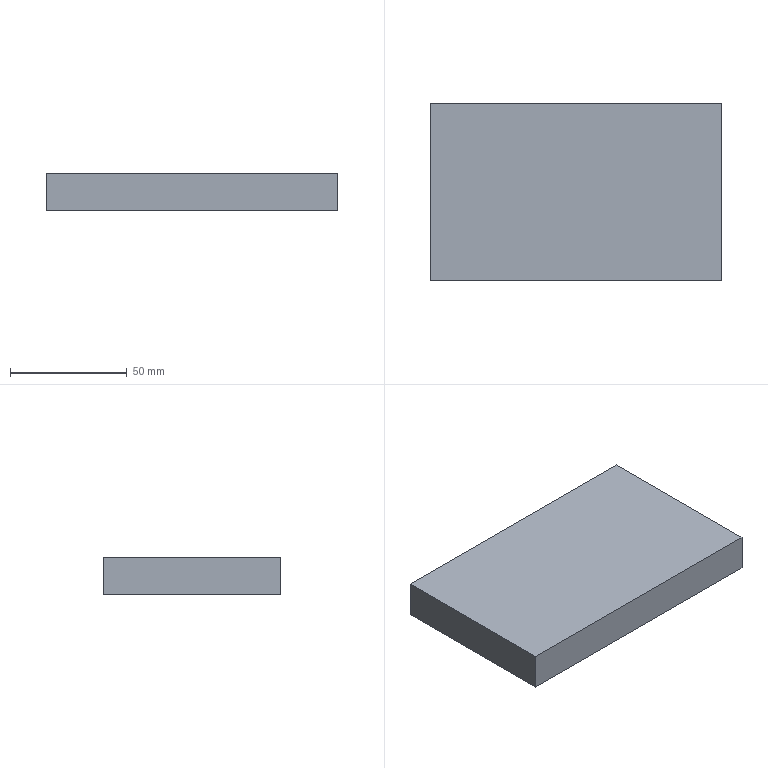Part | SolidWorks | features BaseBody 1 | 1 solid | 6 faces | box 125 x 76.2 x 16 mm | volume 152400 mm3 | plane 6
STEP:
#1=CARTESIAN_POINT('',(-6.214,68.433,16.));
#2=VERTEX_POINT('',#1);
#3=CARTESIAN_POINT('',(-6.214,-7.767,16.));
#4=VERTEX_POINT('',#3);
#5=CARTESIAN_POINT('',(-6.214,30.333,16.));
#6=DIRECTION('',(0.,-1.,0.));
#7=VECTOR('',#6,1000.);
#8=LINE('',#5,#7);
#9=EDGE_CURVE('',#2,#4,#8,.T.);
#10=ORIENTED_EDGE('',*,*,#9,.T.);
#11=CARTESIAN_POINT('',(118.786,-7.767,16.));
#12=VERTEX_POINT('',#11);
#13=CARTESIAN_POINT('',(56.286,-7.767,16.));
#14=DIRECTION('',(1.,0.,0.));
#15=VECTOR('',#14,1000.);
#16=LINE('',#13,#15);
#17=EDGE_CURVE('',#4,#12,#16,.T.);
#18=ORIENTED_EDGE('',*,*,#17,.T.);
#19=CARTESIAN_POINT('',(118.786,68.433,16.));
#20=VERTEX_POINT('',#19);
#21=CARTESIAN_POINT('',(118.786,30.333,16.));
#22=DIRECTION('',(0.,1.,0.));
#23=VECTOR('',#22,1000.);
#24=LINE('',#21,#23);
#25=EDGE_CURVE('',#12,#20,#24,.T.);
#26=ORIENTED_EDGE('',*,*,#25,.T.);
#27=CARTESIAN_POINT('',(56.286,68.433,16.));
#28=DIRECTION('',(-1.,0.,0.));
#29=VECTOR('',#28,1000.);
#30=LINE('',#27,#29);
#31=EDGE_CURVE('',#20,#2,#30,.T.);
#32=ORIENTED_EDGE('',*,*,#31,.T.);
#33=EDGE_LOOP('',(#10,#18,#26,#32));
#34=FACE_OUTER_BOUND('',#33,.T.);
#35=CARTESIAN_POINT('',(56.286,30.333,16.));
#36=DIRECTION('',(0.,0.,1.));
#37=DIRECTION('',(1.,0.,0.));
#38=AXIS2_PLACEMENT_3D('',#35,#36,#37);
#39=PLANE('',#38);
#40=ADVANCED_FACE('',(#34),#39,.T.);
#41=CARTESIAN_POINT('',(-6.214,-7.767,0.));
#42=VERTEX_POINT('',#41);
#43=CARTESIAN_POINT('',(118.786,-7.767,0.));
#44=VERTEX_POINT('',#43);
#45=CARTESIAN_POINT('',(118.786,-7.767,0.));
#46=DIRECTION('',(1.,0.,0.));
#47=VECTOR('',#46,1000.);
#48=LINE('',#45,#47);
#49=EDGE_CURVE('',#42,#44,#48,.T.);
#50=ORIENTED_EDGE('',*,*,#49,.T.);
#51=CARTESIAN_POINT('',(118.786,-7.767,0.));
#52=DIRECTION('',(0.,0.,1.));
#53=VECTOR('',#52,1000.);
#54=LINE('',#51,#53);
#55=EDGE_CURVE('',#44,#12,#54,.T.);
#56=ORIENTED_EDGE('',*,*,#55,.T.);
#57=ORIENTED_EDGE('',*,*,#17,.F.);
#58=CARTESIAN_POINT('',(-6.214,-7.767,0.));
#59=DIRECTION('',(0.,0.,-1.));
#60=VECTOR('',#59,1000.);
#61=LINE('',#58,#60);
#62=EDGE_CURVE('',#4,#42,#61,.T.);
#63=ORIENTED_EDGE('',*,*,#62,.T.);
#64=EDGE_LOOP('',(#50,#56,#57,#63));
#65=FACE_OUTER_BOUND('',#64,.T.);
#66=CARTESIAN_POINT('',(118.786,-7.767,0.));
#67=DIRECTION('',(0.,-1.,0.));
#68=DIRECTION('',(1.,0.,0.));
#69=AXIS2_PLACEMENT_3D('',#66,#67,#68);
#70=PLANE('',#69);
#71=ADVANCED_FACE('',(#65),#70,.T.);
#72=CARTESIAN_POINT('',(-6.214,68.433,0.));
#73=VERTEX_POINT('',#72);
#74=CARTESIAN_POINT('',(-6.214,-7.767,0.));
#75=DIRECTION('',(0.,-1.,0.));
#76=VECTOR('',#75,1000.);
#77=LINE('',#74,#76);
#78=EDGE_CURVE('',#73,#42,#77,.T.);
#79=ORIENTED_EDGE('',*,*,#78,.T.);
#80=ORIENTED_EDGE('',*,*,#62,.F.);
#81=ORIENTED_EDGE('',*,*,#9,.F.);
#82=CARTESIAN_POINT('',(-6.214,68.433,0.));
#83=DIRECTION('',(0.,0.,-1.));
#84=VECTOR('',#83,1000.);
#85=LINE('',#82,#84);
#86=EDGE_CURVE('',#2,#73,#85,.T.);
#87=ORIENTED_EDGE('',*,*,#86,.T.);
#88=EDGE_LOOP('',(#79,#80,#81,#87));
#89=FACE_OUTER_BOUND('',#88,.T.);
#90=CARTESIAN_POINT('',(-6.214,-7.767,0.));
#91=DIRECTION('',(-1.,0.,0.));
#92=DIRECTION('',(0.,-1.,0.));
#93=AXIS2_PLACEMENT_3D('',#90,#91,#92);
#94=PLANE('',#93);
#95=ADVANCED_FACE('',(#89),#94,.T.);
#96=CARTESIAN_POINT('',(118.786,68.433,0.));
#97=VERTEX_POINT('',#96);
#98=CARTESIAN_POINT('',(-6.214,68.433,0.));
#99=DIRECTION('',(-1.,0.,0.));
#100=VECTOR('',#99,1000.);
#101=LINE('',#98,#100);
#102=EDGE_CURVE('',#97,#73,#101,.T.);
#103=ORIENTED_EDGE('',*,*,#102,.T.);
#104=ORIENTED_EDGE('',*,*,#86,.F.);
#105=ORIENTED_EDGE('',*,*,#31,.F.);
#106=CARTESIAN_POINT('',(118.786,68.433,0.));
#107=DIRECTION('',(0.,0.,-1.));
#108=VECTOR('',#107,1000.);
#109=LINE('',#106,#108);
#110=EDGE_CURVE('',#20,#97,#109,.T.);
#111=ORIENTED_EDGE('',*,*,#110,.T.);
#112=EDGE_LOOP('',(#103,#104,#105,#111));
#113=FACE_OUTER_BOUND('',#112,.T.);
#114=CARTESIAN_POINT('',(-6.214,68.433,0.));
#115=DIRECTION('',(0.,1.,0.));
#116=DIRECTION('',(0.,0.,1.));
#117=AXIS2_PLACEMENT_3D('',#114,#115,#116);
#118=PLANE('',#117);
#119=ADVANCED_FACE('',(#113),#118,.T.);
#120=CARTESIAN_POINT('',(118.786,68.433,0.));
#121=DIRECTION('',(0.,1.,0.));
#122=VECTOR('',#121,1000.);
#123=LINE('',#120,#122);
#124=EDGE_CURVE('',#44,#97,#123,.T.);
#125=ORIENTED_EDGE('',*,*,#124,.T.);
#126=ORIENTED_EDGE('',*,*,#110,.F.);
#127=ORIENTED_EDGE('',*,*,#25,.F.);
#128=ORIENTED_EDGE('',*,*,#55,.F.);
#129=EDGE_LOOP('',(#125,#126,#127,#128));
#130=FACE_OUTER_BOUND('',#129,.T.);
#131=CARTESIAN_POINT('',(118.786,68.433,0.));
#132=DIRECTION('',(1.,0.,0.));
#133=DIRECTION('',(0.,0.,-1.));
#134=AXIS2_PLACEMENT_3D('',#131,#132,#133);
#135=PLANE('',#134);
#136=ADVANCED_FACE('',(#130),#135,.T.);
#137=ORIENTED_EDGE('',*,*,#124,.F.);
#138=ORIENTED_EDGE('',*,*,#49,.F.);
#139=ORIENTED_EDGE('',*,*,#78,.F.);
#140=ORIENTED_EDGE('',*,*,#102,.F.);
#141=EDGE_LOOP('',(#137,#138,#139,#140));
#142=FACE_OUTER_BOUND('',#141,.T.);
#143=CARTESIAN_POINT('',(56.286,30.333,0.));
#144=DIRECTION('',(0.,0.,1.));
#145=DIRECTION('',(1.,0.,0.));
#146=AXIS2_PLACEMENT_3D('',#143,#144,#145);
#147=PLANE('',#146);
#148=ADVANCED_FACE('',(#142),#147,.F.);
#149=CLOSED_SHELL('',(#40,#71,#95,#119,#136,#148));
#150=MANIFOLD_SOLID_BREP('',#149);
#151=CARTESIAN_POINT('',(0.,0.,0.));
#152=DIRECTION('',(0.,0.,1.));
#153=DIRECTION('',(1.,0.,0.));
#154=AXIS2_PLACEMENT_3D('',#151,#152,#153);
#155=(LENGTH_UNIT()NAMED_UNIT(*)SI_UNIT(.MILLI.,.METRE.));
#156=UNCERTAINTY_MEASURE_WITH_UNIT(LENGTH_MEASURE(0.00001),#155,'','');
#157=(NAMED_UNIT(*)PLANE_ANGLE_UNIT()SI_UNIT($,.RADIAN.));
#158=(NAMED_UNIT(*)SI_UNIT($,.STERADIAN.)SOLID_ANGLE_UNIT());
#159=(GEOMETRIC_REPRESENTATION_CONTEXT(3)GLOBAL_UNCERTAINTY_ASSIGNED_CONTEXT((#156))GLOBAL_UNIT_ASSIGNED_CONTEXT((#155,#157,#158))REPRESENTATION_CONTEXT('',''));
#160=ADVANCED_BREP_SHAPE_REPRESENTATION('',(#150,#154),#159);